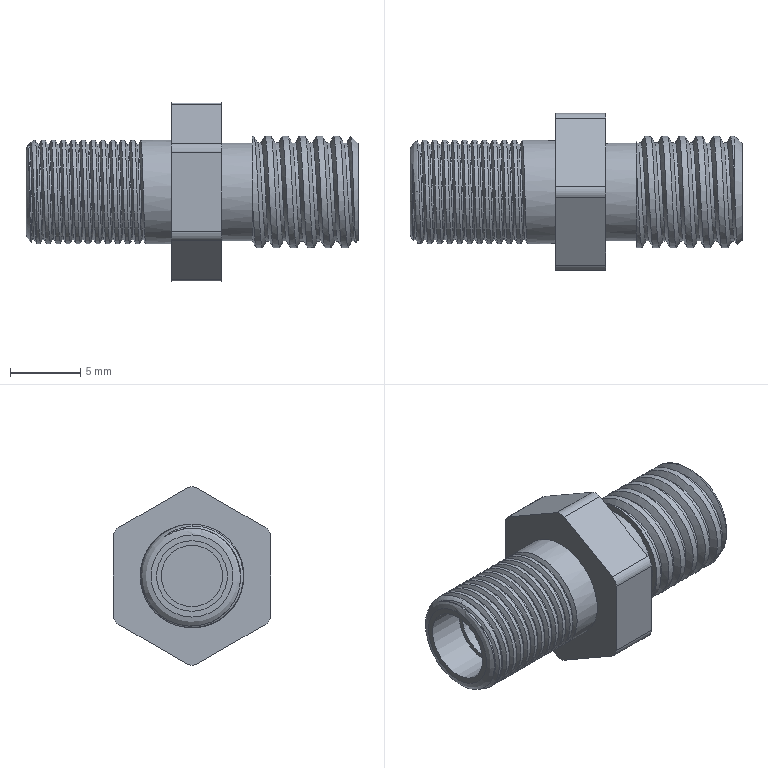Part | NX | features solid 2 | 1 solid | 48 faces | box 23.597 x 11.176 x 12.669 mm | volume 899.752 mm3 | cylinder 25 | plane 16 | spline 4 | torus 2 | cone 1 | commonest cylinder face diameters 7.366 x12 1.524 x6 4.369 x2 5.029 x1 6.807 x1 6.96 x1